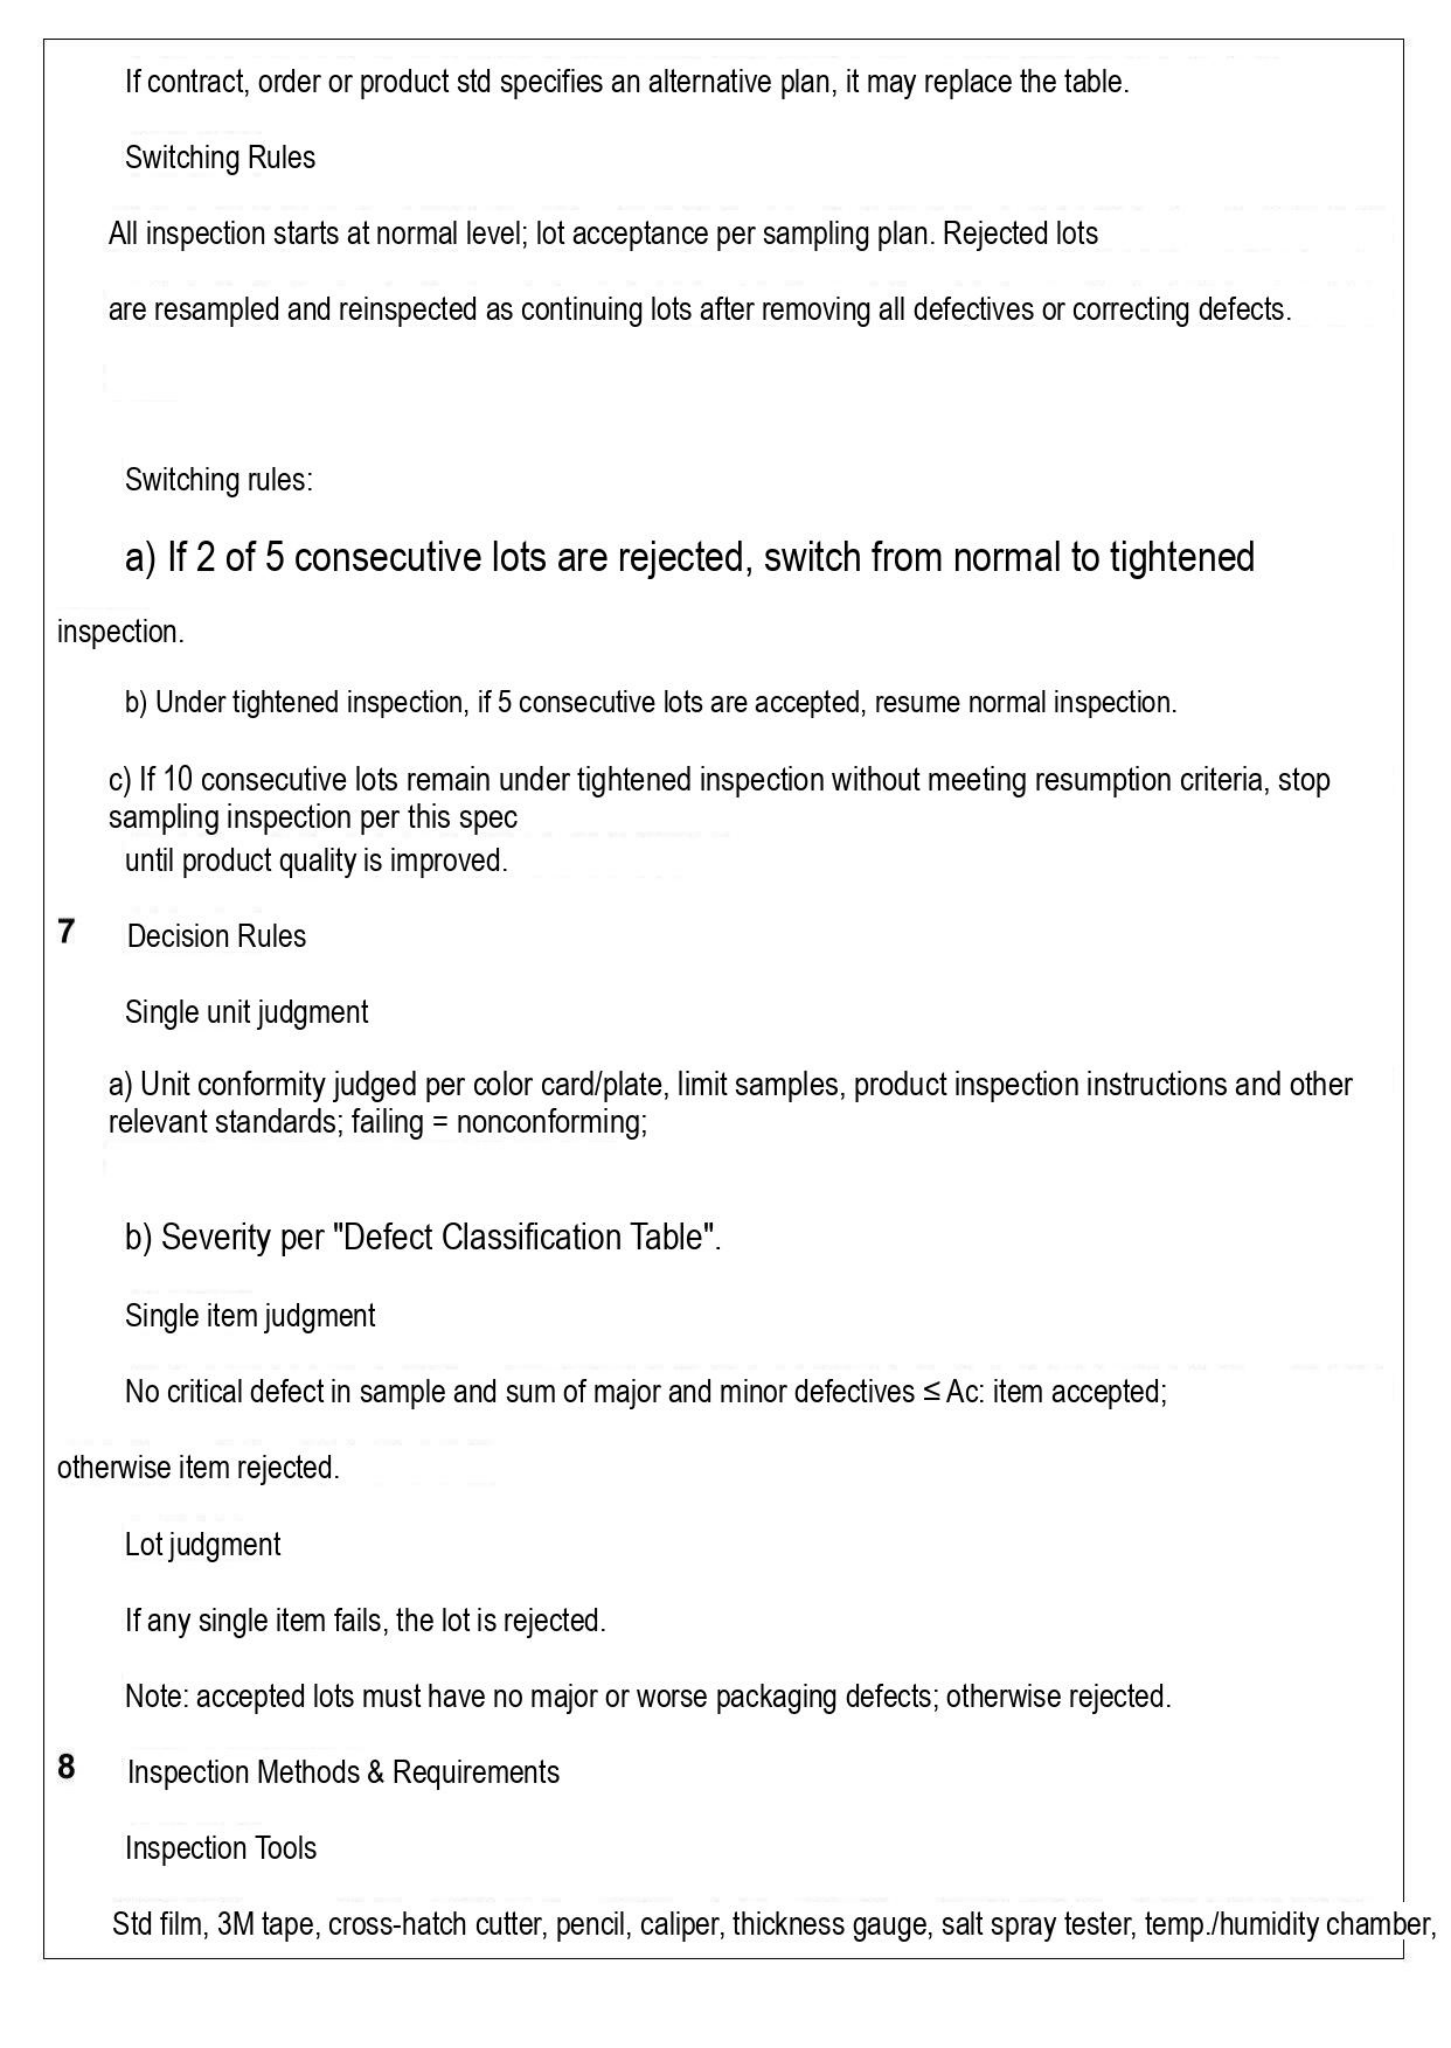If contract, order or product std specifies an alternative plan, it may replace the table.

Switching Rules

All inspection starts at normal level; lot acceptance per sampling plan. Rejected lots

are resampled and reinspected as continuing lots after removing all defectives or correcting defects.

Switching rules:

a) If 2 of 5 consecutive lots are rejected, switch from normal to tightened

inspection.

b) Under tightened inspection, if 5 consecutive lots are accepted, resume normal inspection.

c) If 10 consecutive lots remain under tightened inspection without meeting resumption criteria, stop sampling inspection per this spec
until product quality is improved.

7 Decision Rules

Single unit judgment

a) Unit conformity judged per color card/plate, limit samples, product inspection instructions and other relevant standards; failing = nonconforming;

b) Severity per "Defect Classification Table".

Single item judgment

No critical defect in sample and sum of major and minor defectives ≤ Ac: item accepted;

otherwise item rejected.

Lot judgment

If any single item fails, the lot is rejected.

Note: accepted lots must have no major or worse packaging defects; otherwise rejected.

8 Inspection Methods & Requirements

Inspection Tools

Std film, 3M tape, cross-hatch cutter, pencil, caliper, thickness gauge, salt spray tester, temp./humidity chamber,
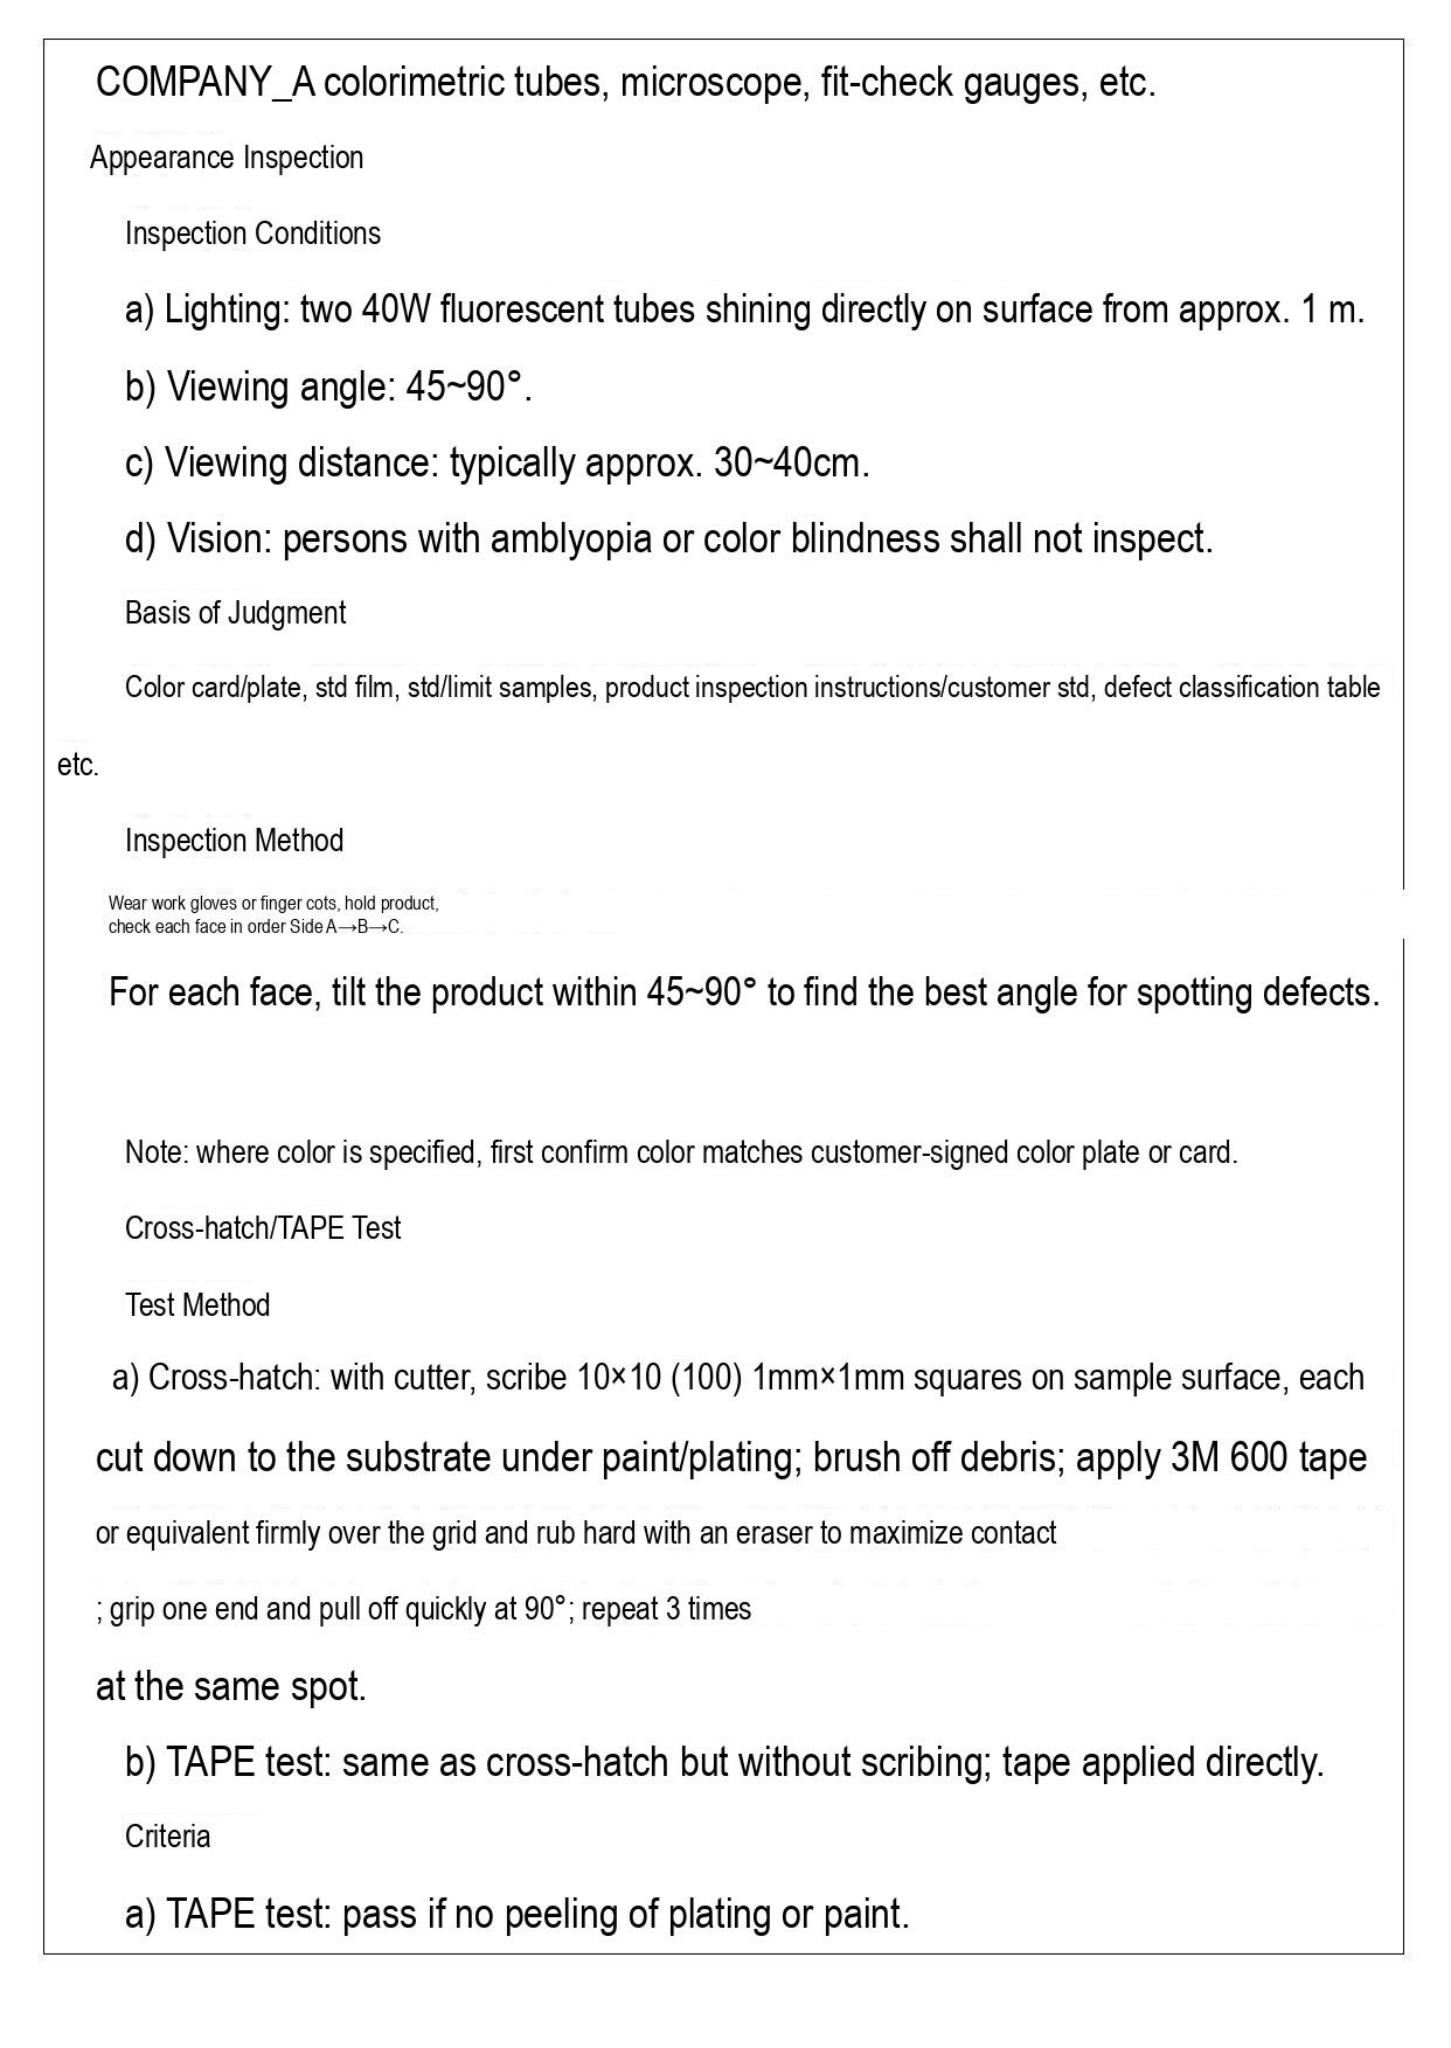COMPANY_A colorimetric tubes, microscope, fit-check gauges, etc.

Appearance Inspection

Inspection Conditions

a) Lighting: two 40W fluorescent tubes shining directly on surface from approx. 1 m.

b) Viewing angle: 45~90°.

c) Viewing distance: typically approx. 30~40cm.

d) Vision: persons with amblyopia or color blindness shall not inspect.

Basis of Judgment

Color card/plate, std film, std/limit samples, product inspection instructions/customer std, defect classification table etc.

Inspection Method

Wear work gloves or finger cots, hold product, check each face in order Side A→B→C.

For each face, tilt the product within 45~90° to find the best angle for spotting defects.

Note: where color is specified, first confirm color matches customer-signed color plate or card.

Cross-hatch/TAPE Test

Test Method

a) Cross-hatch: with cutter, scribe 10×10 (100) 1mm×1mm squares on sample surface, each cut down to the substrate under paint/plating; brush off debris; apply 3M 600 tape or equivalent firmly over the grid and rub hard with an eraser to maximize contact; grip one end and pull off quickly at 90°; repeat 3 times at the same spot.

b) TAPE test: same as cross-hatch but without scribing; tape applied directly.

Criteria

a) TAPE test: pass if no peeling of plating or paint.
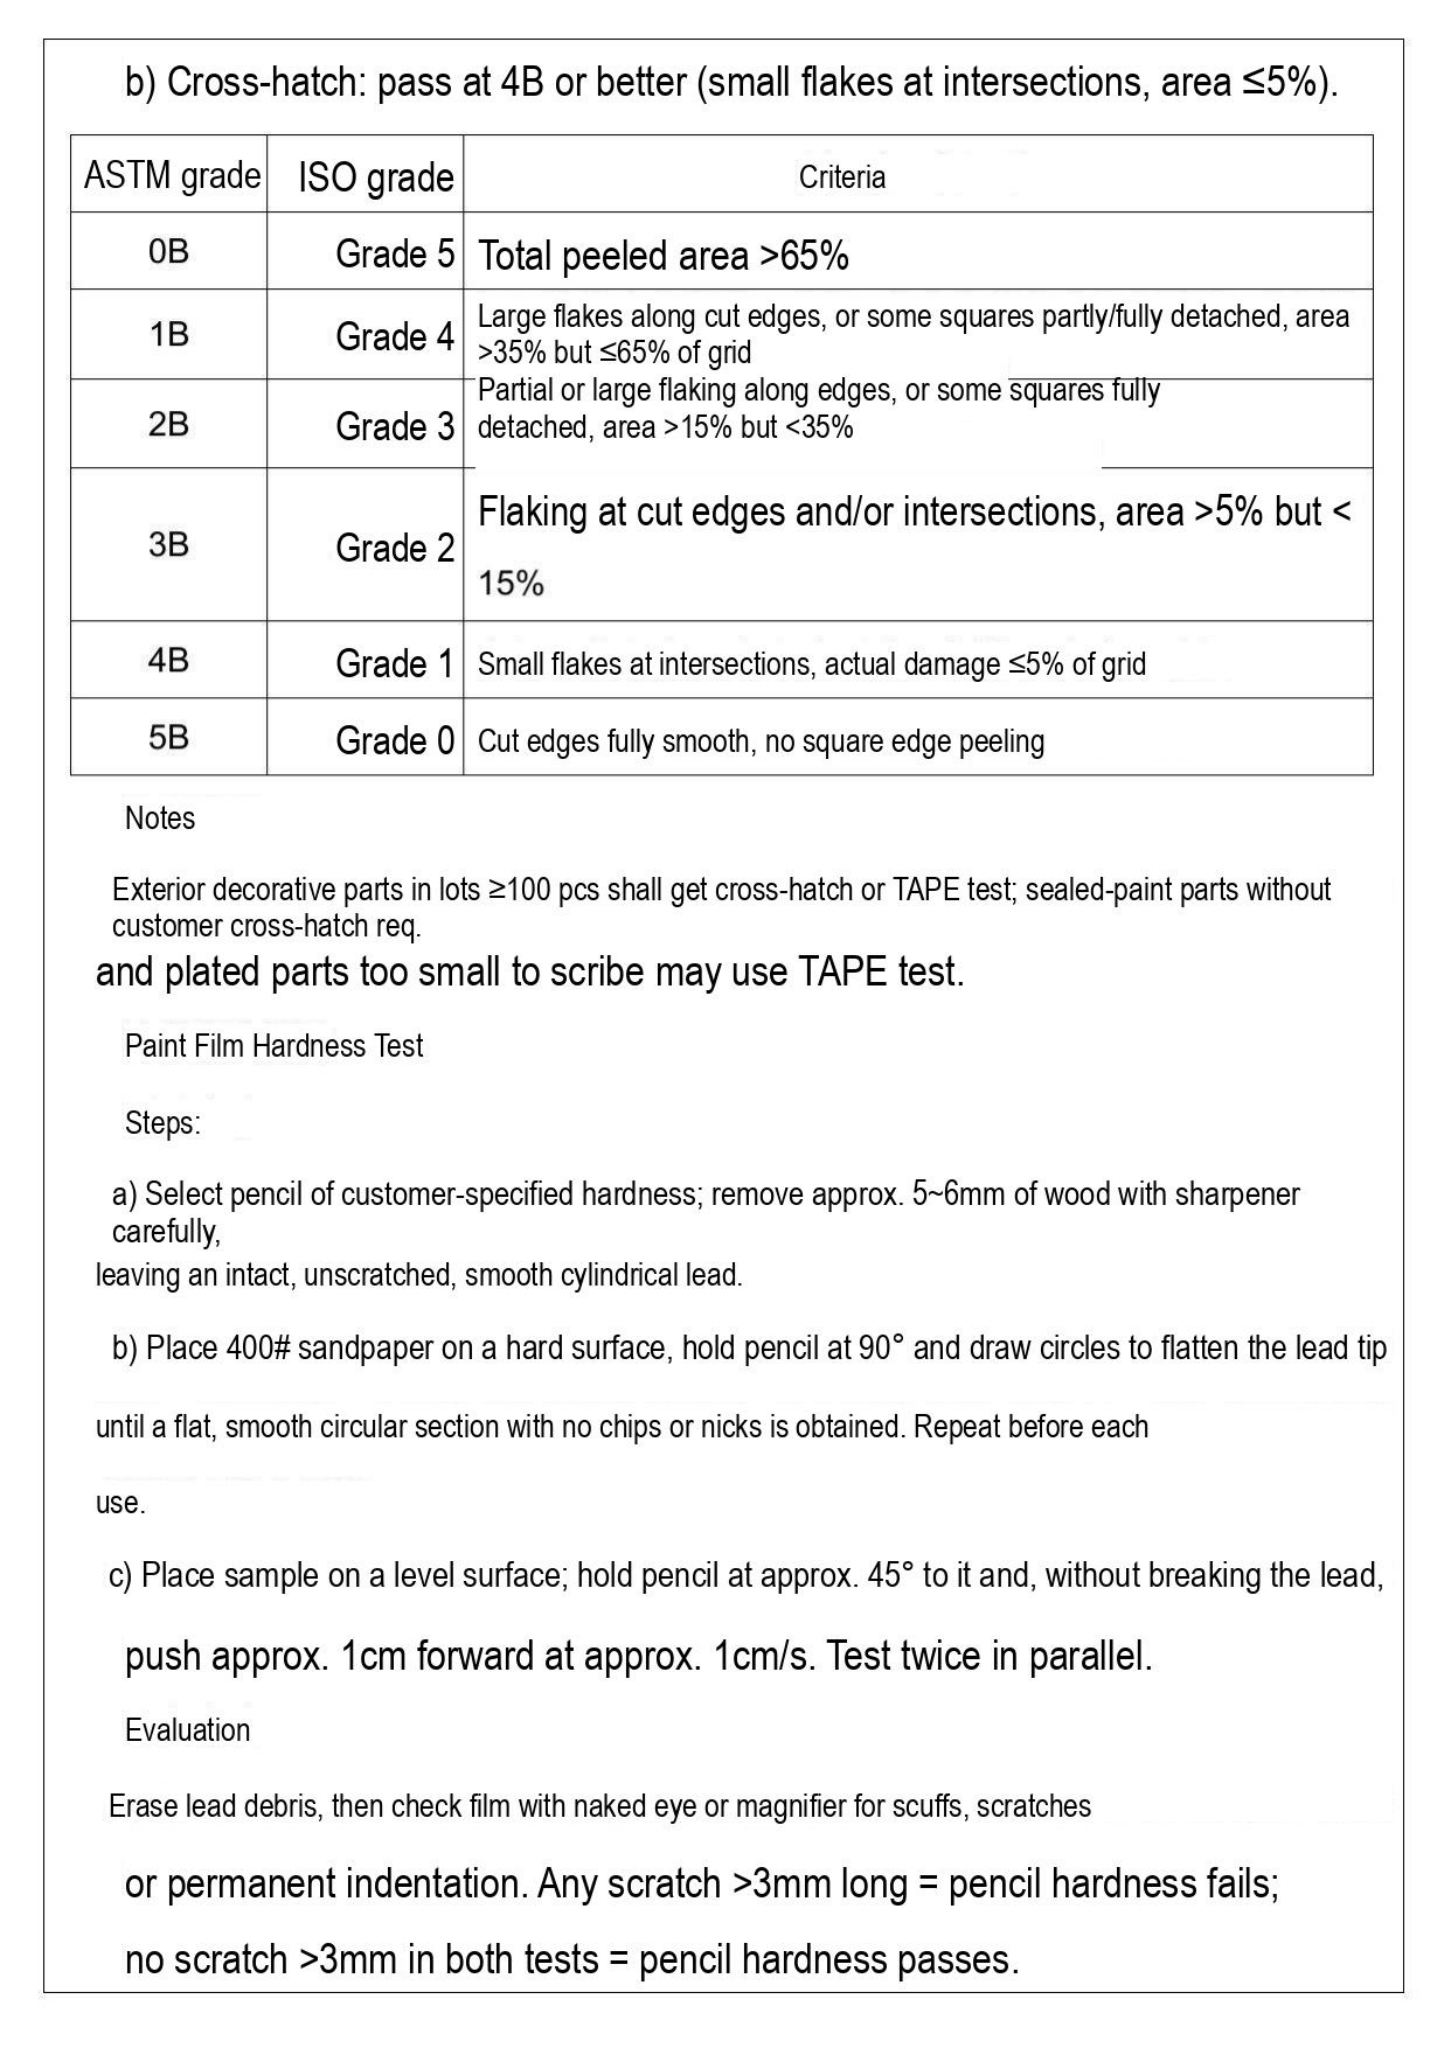b) Cross-hatch: pass at 4B or better (small flakes at intersections, area ≤5%).

| ASTM grade | ISO grade | Criteria |
|---|---|---|
| 0B | Grade 5 | Total peeled area >65% |
| 1B | Grade 4 | Large flakes along cut edges, or some squares partly/fully detached, area >35% but ≤65% of grid |
| 2B | Grade 3 | Partial or large flaking along edges, or some squares fully detached, area >15% but <35% |
| 3B | Grade 2 | Flaking at cut edges and/or intersections, area >5% but < 15% |
| 4B | Grade 1 | Small flakes at intersections, actual damage ≤5% of grid |
| 5B | Grade 0 | Cut edges fully smooth, no square edge peeling |

Notes

Exterior decorative parts in lots ≥100 pcs shall get cross-hatch or TAPE test; sealed-paint parts without customer cross-hatch req.
and plated parts too small to scribe may use TAPE test.

Paint Film Hardness Test

Steps:

a) Select pencil of customer-specified hardness; remove approx. 5~6mm of wood with sharpener carefully,
leaving an intact, unscratched, smooth cylindrical lead.

b) Place 400# sandpaper on a hard surface, hold pencil at 90° and draw circles to flatten the lead tip
until a flat, smooth circular section with no chips or nicks is obtained. Repeat before each
use.

c) Place sample on a level surface; hold pencil at approx. 45° to it and, without breaking the lead,
push approx. 1cm forward at approx. 1cm/s. Test twice in parallel.

Evaluation

Erase lead debris, then check film with naked eye or magnifier for scuffs, scratches
or permanent indentation. Any scratch >3mm long = pencil hardness fails;
no scratch >3mm in both tests = pencil hardness passes.
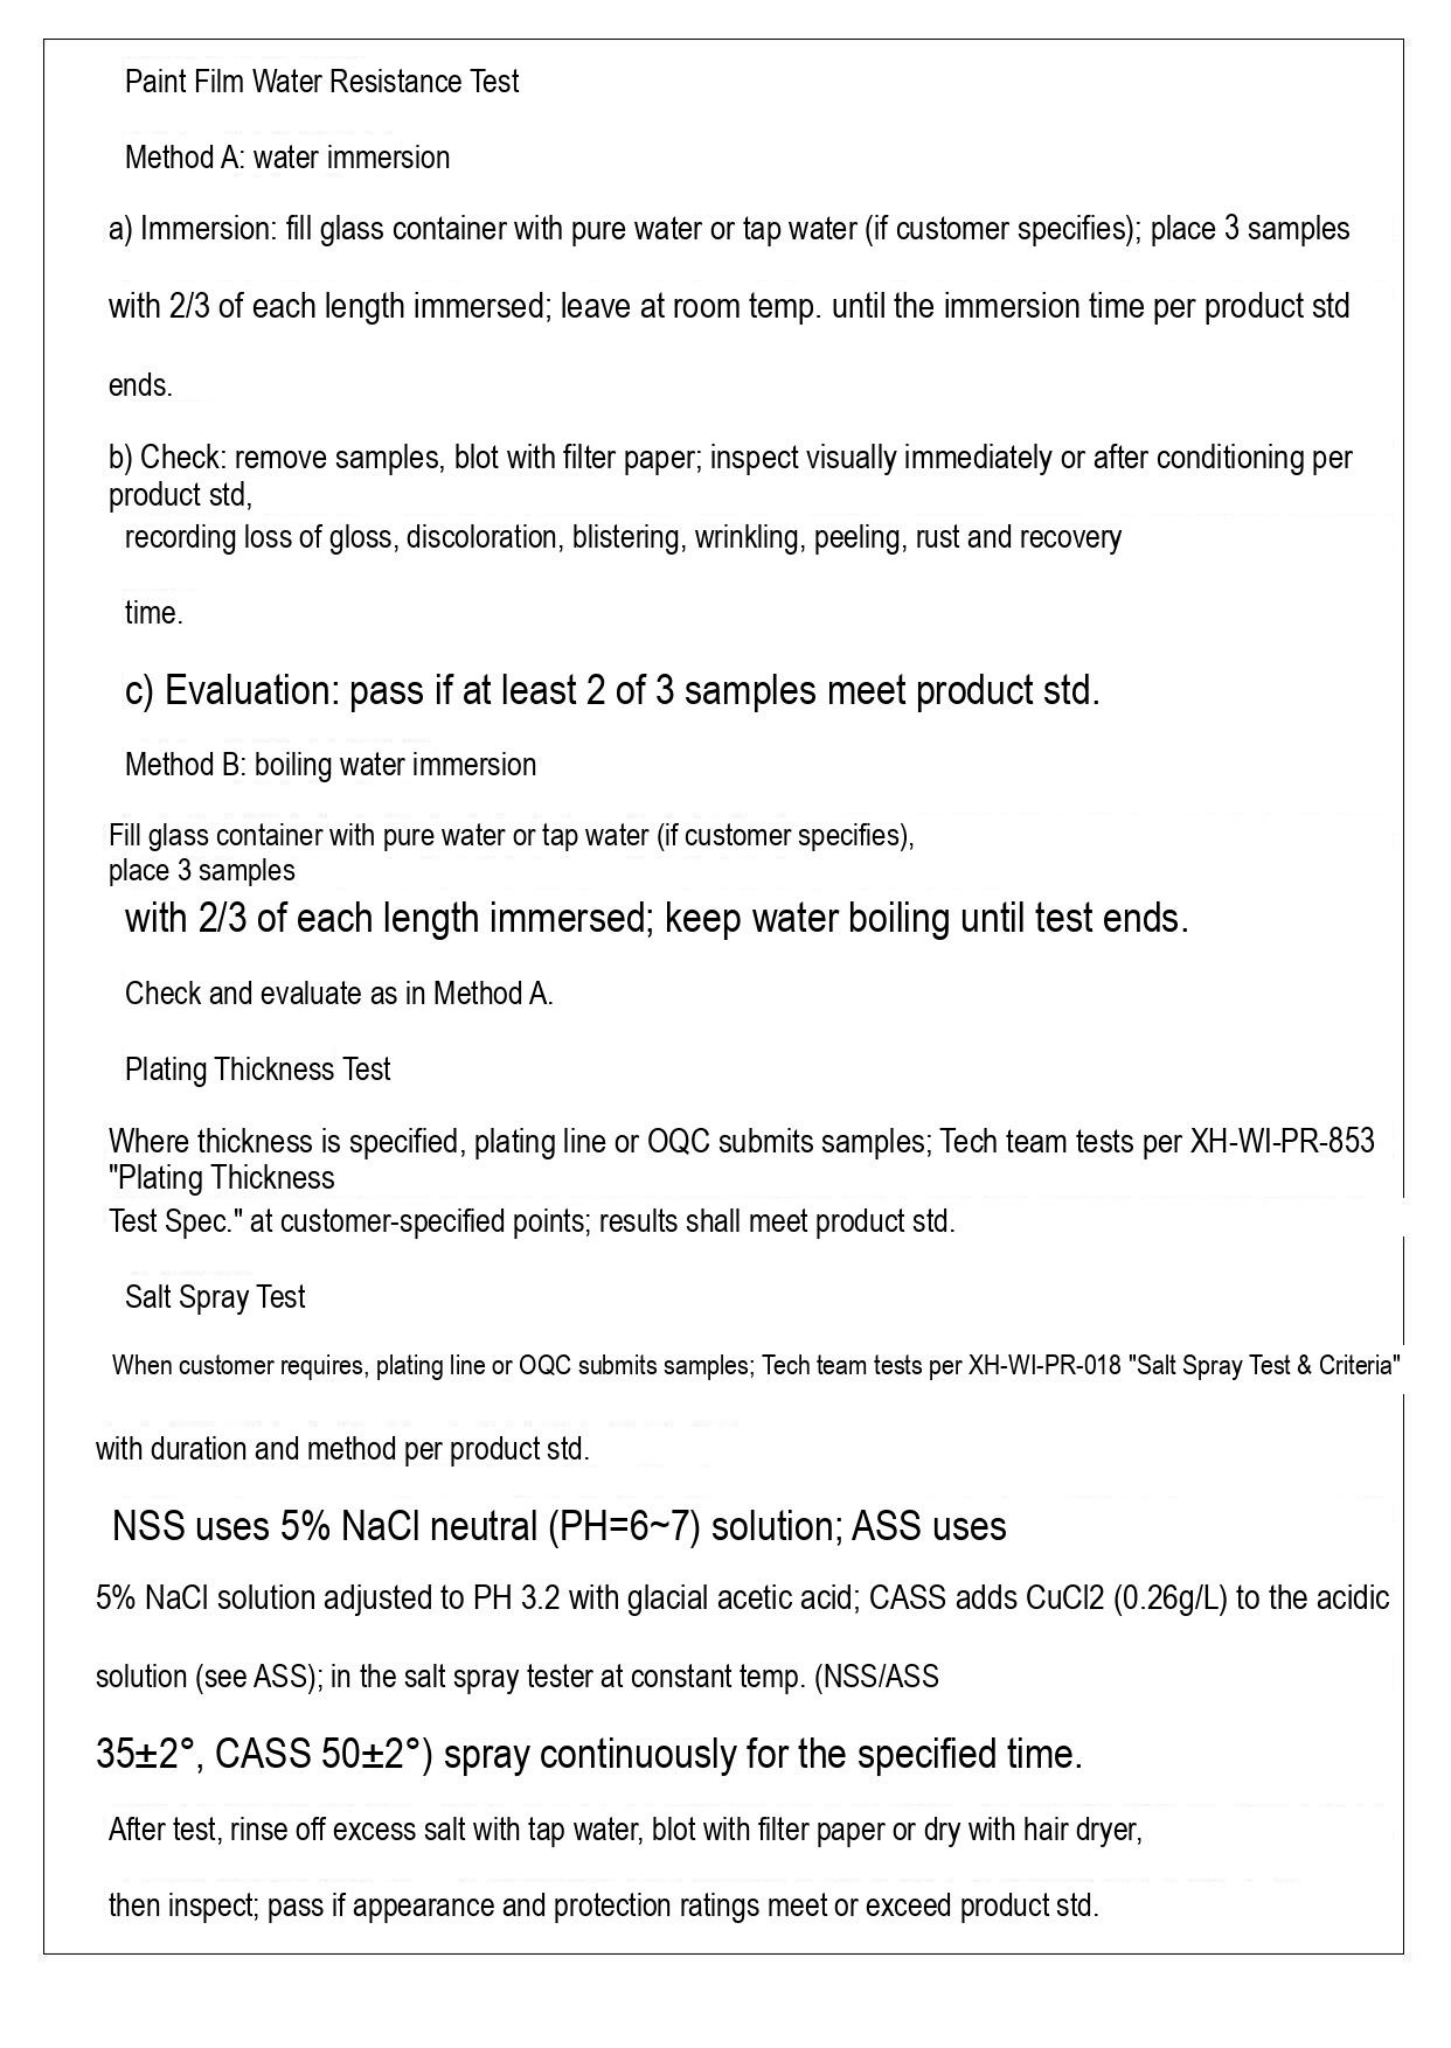Paint Film Water Resistance Test

Method A: water immersion

a) Immersion: fill glass container with pure water or tap water (if customer specifies); place 3 samples

with 2/3 of each length immersed; leave at room temp. until the immersion time per product std

ends.

b) Check: remove samples, blot with filter paper; inspect visually immediately or after conditioning per product std,

recording loss of gloss, discoloration, blistering, wrinkling, peeling, rust and recovery

time.

c) Evaluation: pass if at least 2 of 3 samples meet product std.

Method B: boiling water immersion

Fill glass container with pure water or tap water (if customer specifies), place 3 samples

with 2/3 of each length immersed; keep water boiling until test ends.

Check and evaluate as in Method A.

Plating Thickness Test

Where thickness is specified, plating line or OQC submits samples; Tech team tests per XH-WI-PR-853 "Plating Thickness

Test Spec." at customer-specified points; results shall meet product std.

Salt Spray Test

When customer requires, plating line or OQC submits samples; Tech team tests per XH-WI-PR-018 "Salt Spray Test & Criteria"

with duration and method per product std.

NSS uses 5% NaCl neutral (PH=6~7) solution; ASS uses

5% NaCl solution adjusted to PH 3.2 with glacial acetic acid; CASS adds CuCl2 (0.26g/L) to the acidic

solution (see ASS); in the salt spray tester at constant temp. (NSS/ASS

35±2°, CASS 50±2°) spray continuously for the specified time.

After test, rinse off excess salt with tap water, blot with filter paper or dry with hair dryer,

then inspect; pass if appearance and protection ratings meet or exceed product std.
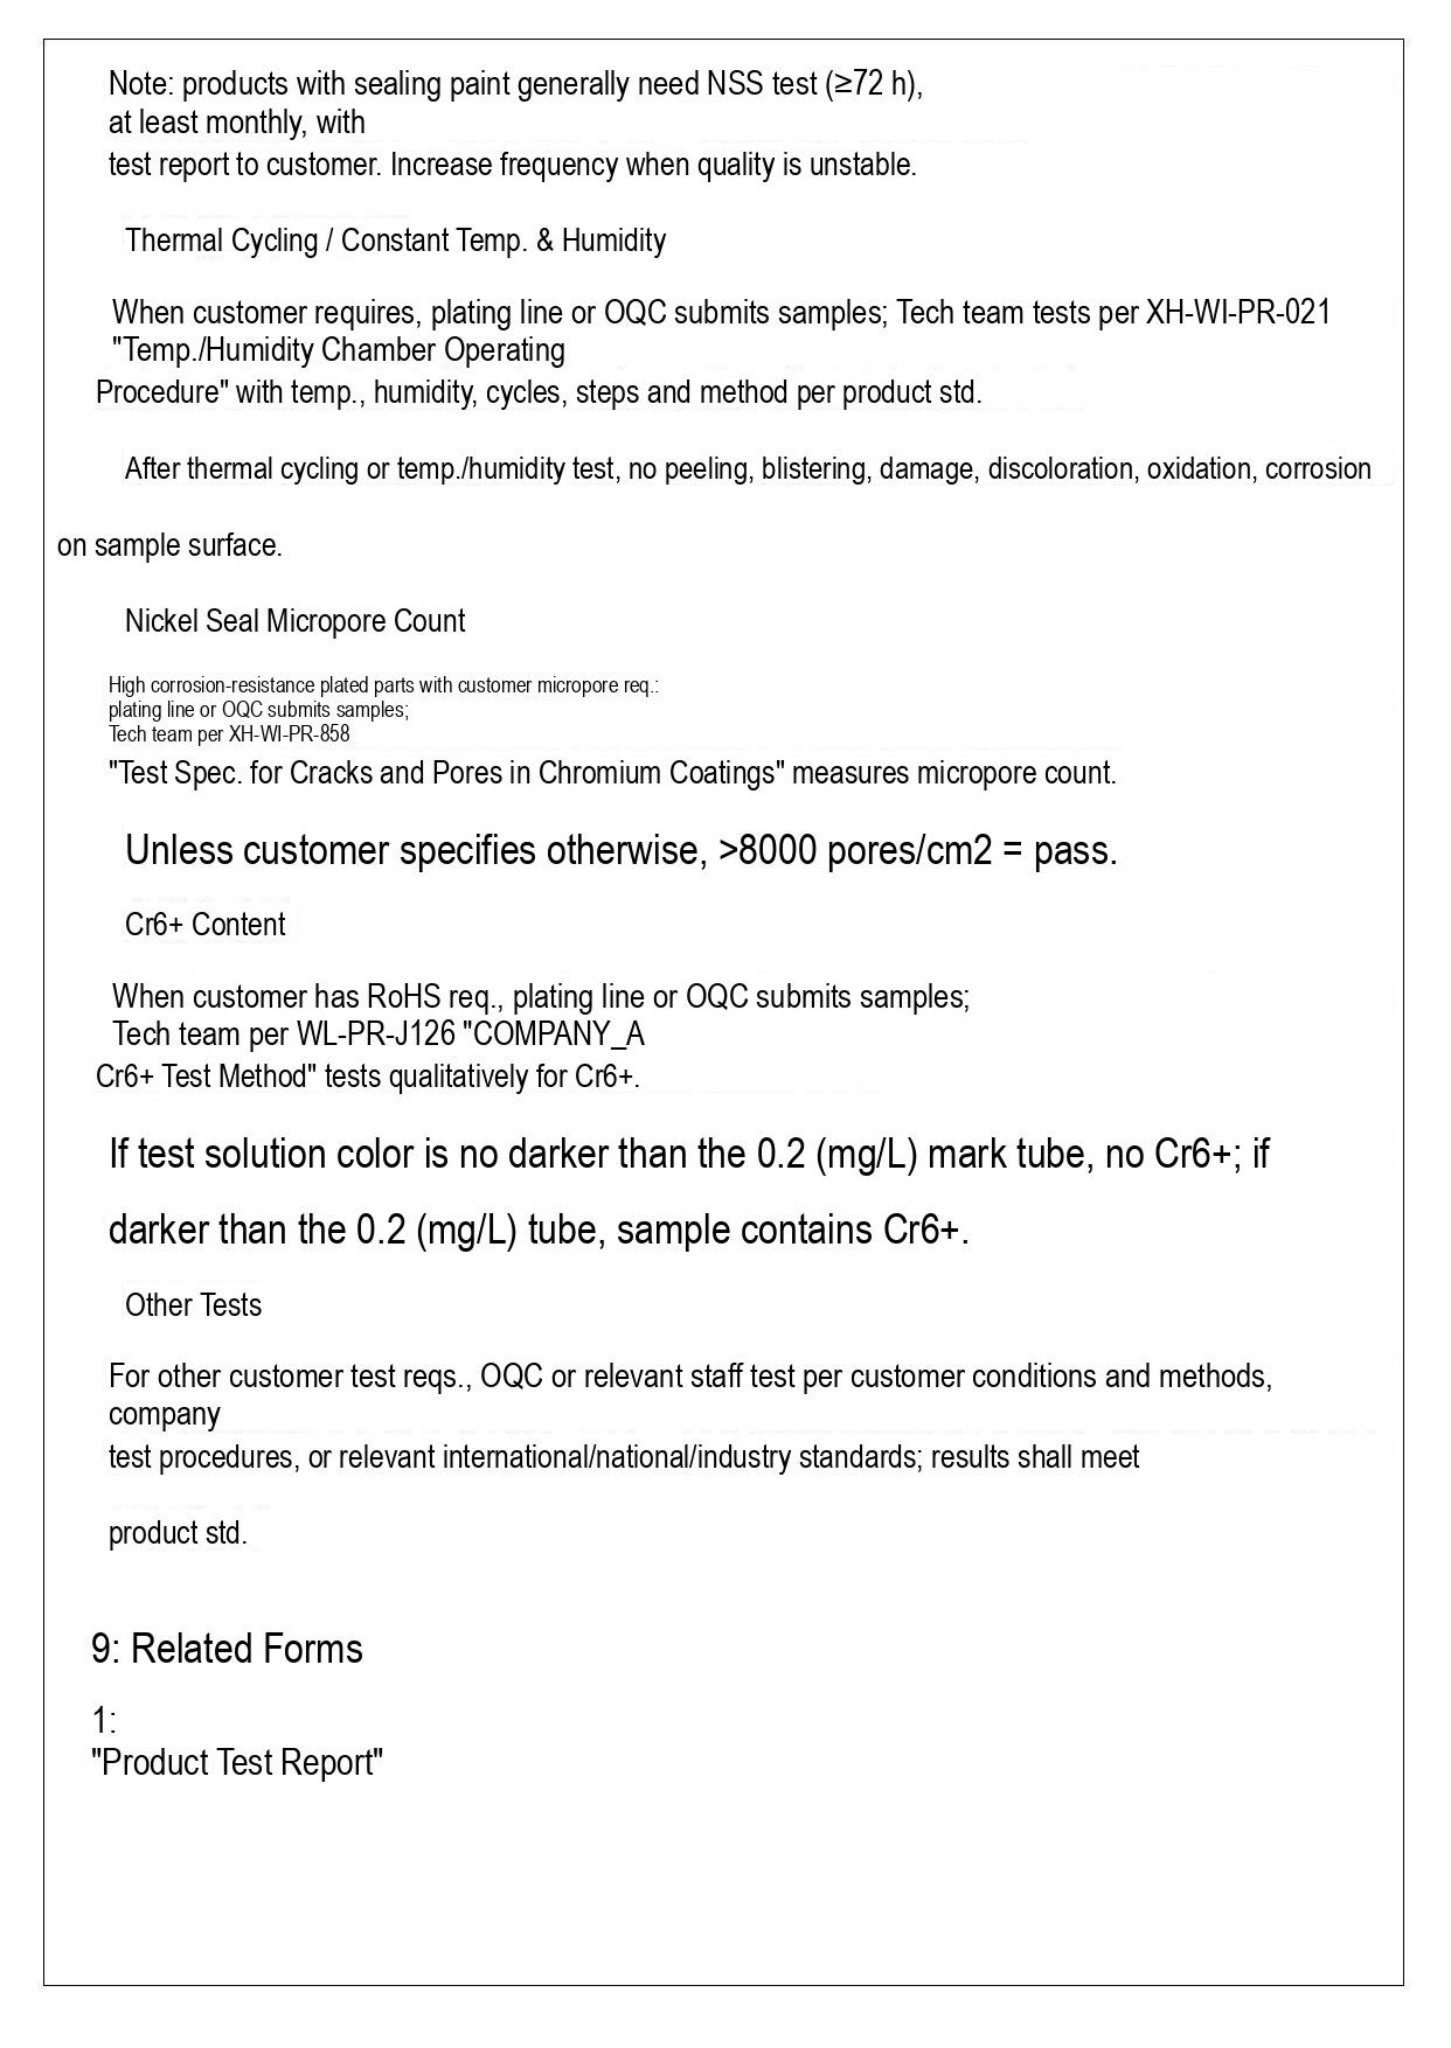Note: products with sealing paint generally need NSS test (≥72 h),
at least monthly, with
test report to customer. Increase frequency when quality is unstable.

Thermal Cycling / Constant Temp. & Humidity

When customer requires, plating line or OQC submits samples; Tech team tests per XH-WI-PR-021 "Temp./Humidity Chamber Operating
Procedure" with temp., humidity, cycles, steps and method per product std.

After thermal cycling or temp./humidity test, no peeling, blistering, damage, discoloration, oxidation, corrosion

on sample surface.

Nickel Seal Micropore Count

High corrosion-resistance plated parts with customer micropore req.:
plating line or OQC submits samples;
Tech team per XH-WI-PR-858
"Test Spec. for Cracks and Pores in Chromium Coatings" measures micropore count.

Unless customer specifies otherwise, >8000 pores/cm2 = pass.

Cr6+ Content

When customer has RoHS req., plating line or OQC submits samples;
Tech team per WL-PR-J126 "COMPANY_A
Cr6+ Test Method" tests qualitatively for Cr6+.

If test solution color is no darker than the 0.2 (mg/L) mark tube, no Cr6+; if

darker than the 0.2 (mg/L) tube, sample contains Cr6+.

Other Tests

For other customer test reqs., OQC or relevant staff test per customer conditions and methods, company
test procedures, or relevant international/national/industry standards; results shall meet

product std.

9: Related Forms

1:
"Product Test Report"